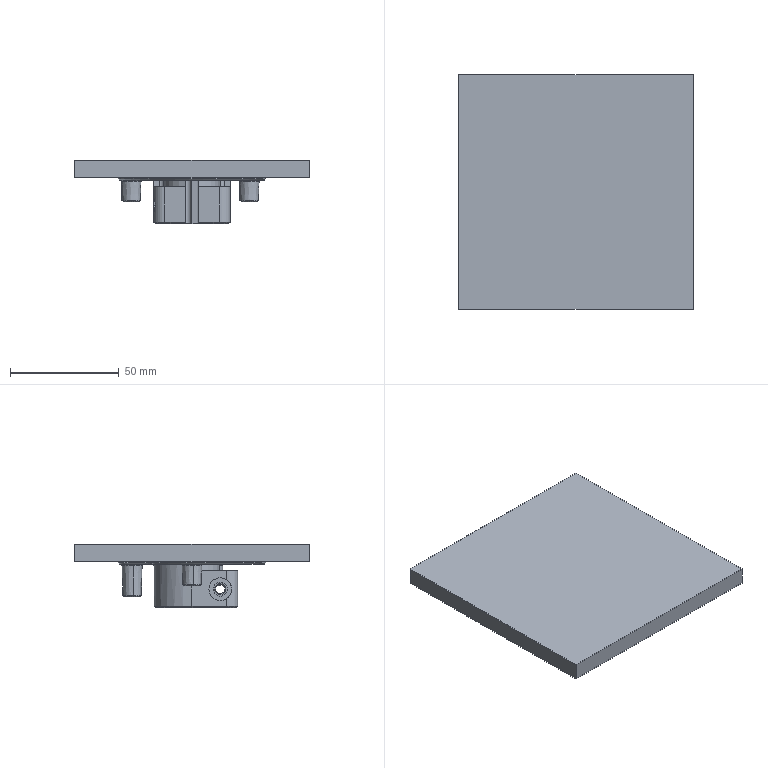Part | 2 solids | 123 faces | box 108 x 108 x 29 mm | volume 107274 mm3 | plane 43 | cone 37 | cylinder 37 | torus 6 | commonest cylinder face diameters 5.1 x6 10 x6 4 x4 6 x4 4.2 x2 6.5 x2